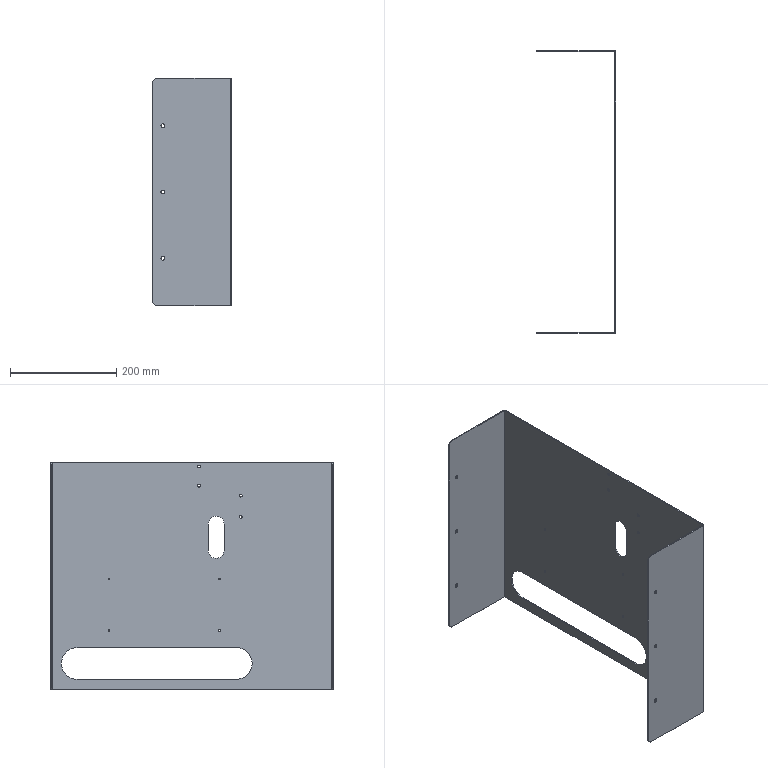Part | SolidWorks | features Cut 2, HoleWzd 2, Fillet 1, FlatPattern 1, ICE 1, LPattern 1, SMBaseFlange 1, SheetMetal 1 | 1 solid | 63 faces | box 150 x 533 x 430 mm | volume 664905 mm3 | cylinder 41 | plane 22 | commonest cylinder face diameters 7 x12 5 x10 3.3 x8 20 x4 60 x3 1 x2